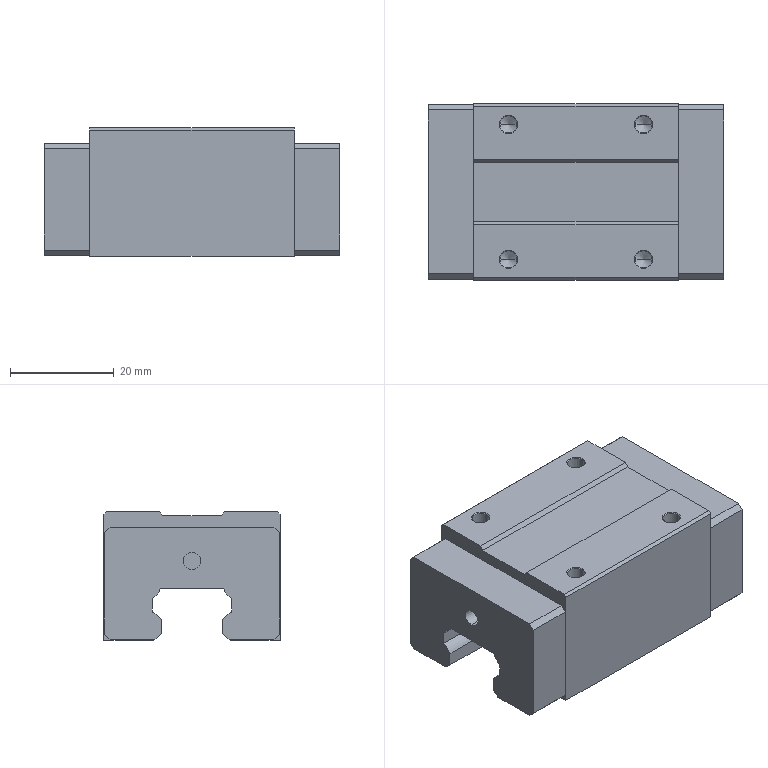Part | SolidWorks | features BaseBody 1 | 1 solid | 90 faces | box 56.9 x 34 x 24.8 mm | volume 37620 mm3 | plane 54 | cylinder 20 | cone 16 | commonest cylinder face diameters 3.3 x12 5.956 x8